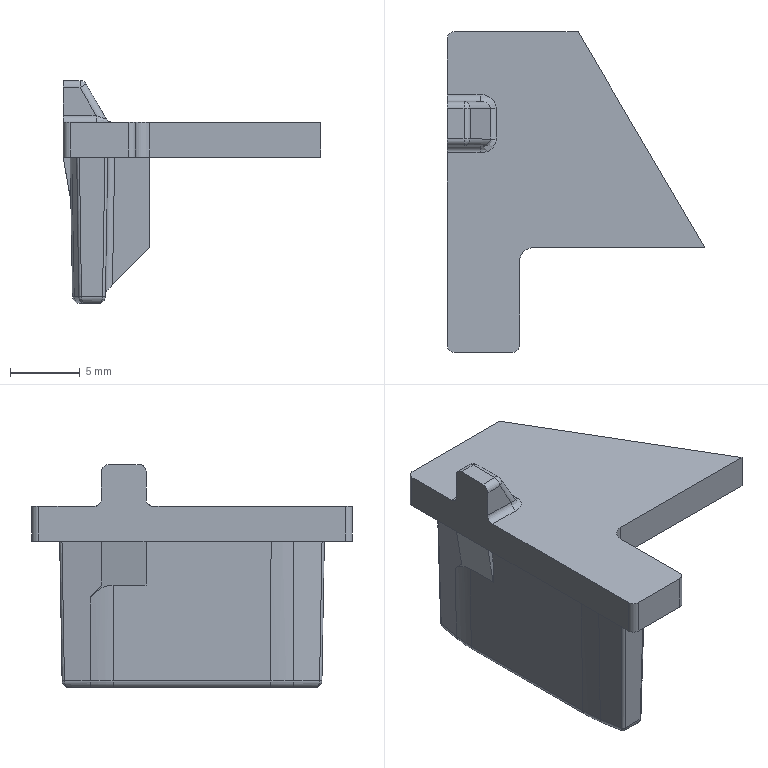Part | STEP file | DZH_7_1 | 1 solid | 69 faces | box 18.5 x 23 x 16 mm | volume 1219 mm3 | plane 31 | cylinder 28 | spline 6 | torus 2 | sphere 2 | commonest cylinder face diameters 1 x21 0.4 x4 20 x2 2 x1